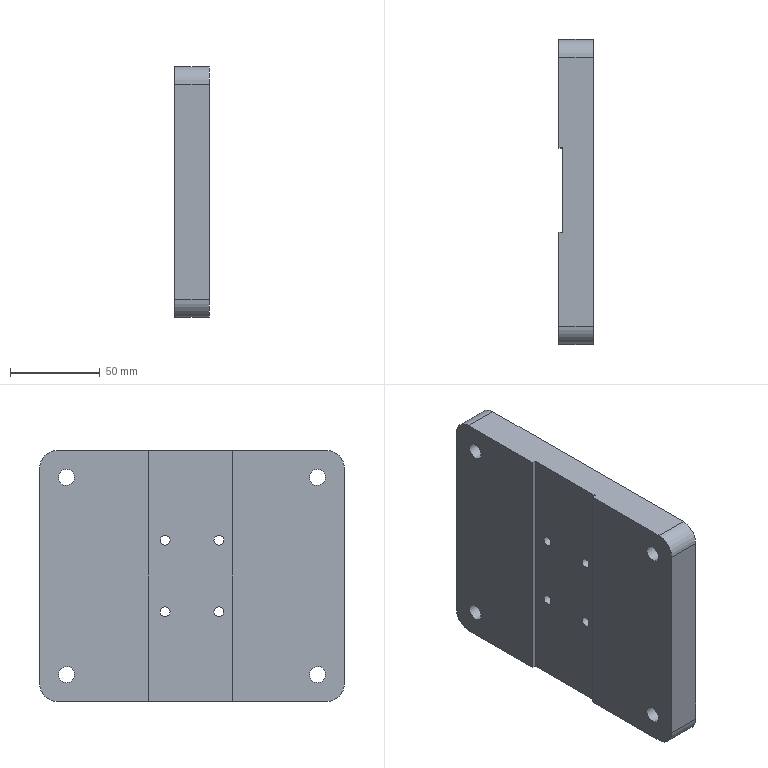Part | STEP file | SN10_013_001_PLACA | 1 solid | 30 faces | box 19 x 170 x 140 mm | volume 426435 mm3 | cylinder 16 | plane 14 | commonest cylinder face diameters 5.5 x4 9 x4 15 x4 20 x4